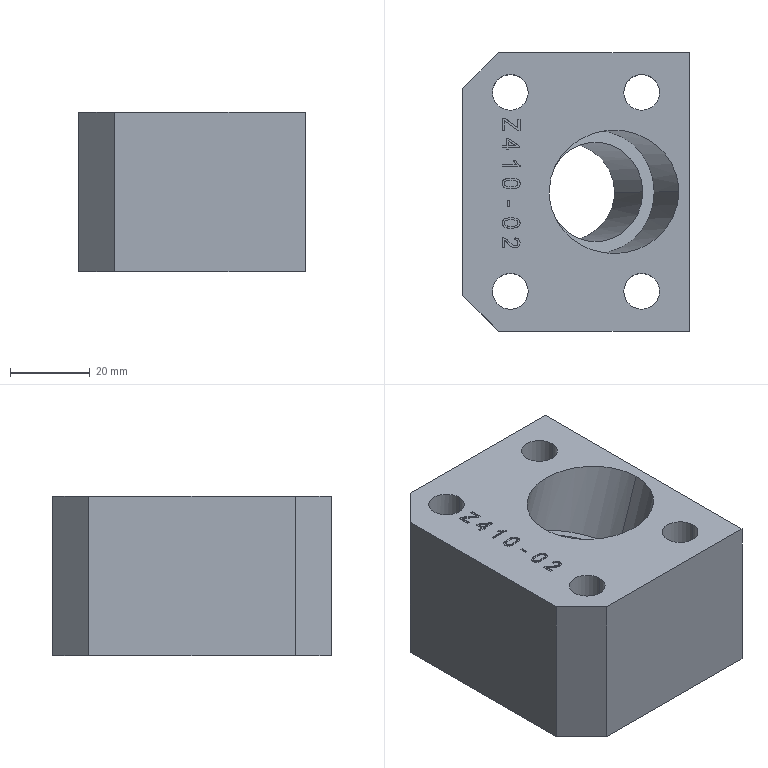Part | Creo | 1 solid | 144 faces | box 57 x 70 x 40 mm | volume 118317 mm3 | other 67 | plane 55 | cylinder 22 | commonest cylinder face diameters 9 x8 14 x8 25 x2 31 x2 3.854 x1 60.776 x1